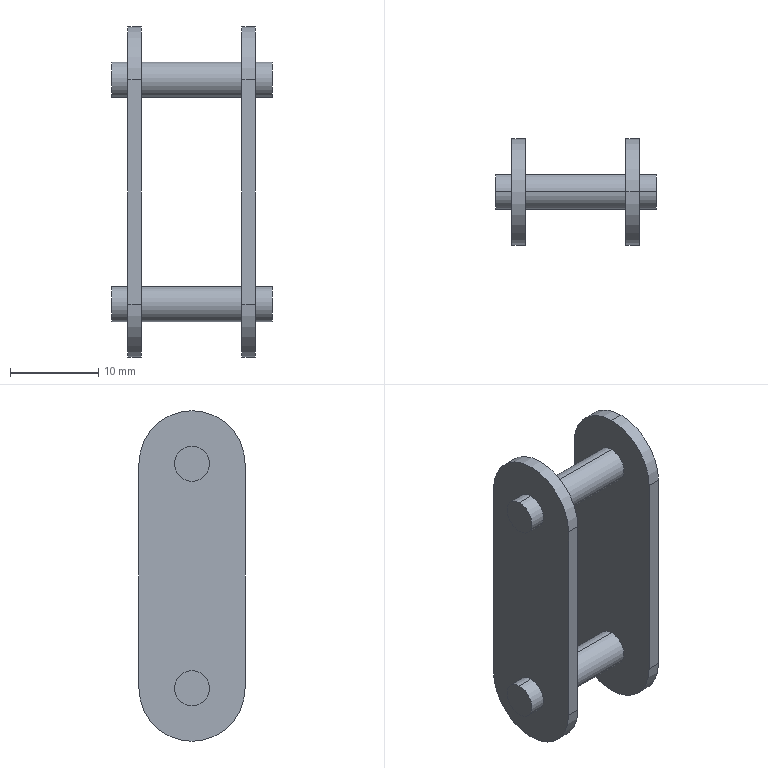Part | STEP file | 0228_Z_Chain_RF2040SSS-441 | 1 solid | 30 faces | box 18.2 x 12 x 37.4 mm | volume 1630 mm3 | cylinder 18 | plane 12 | commonest cylinder face diameters 3.97 x12 12 x6